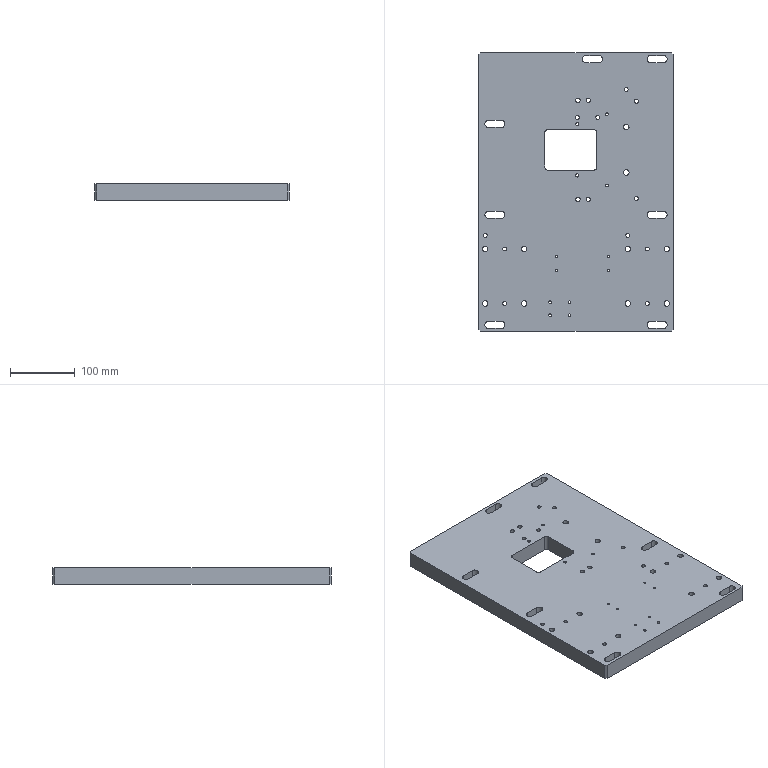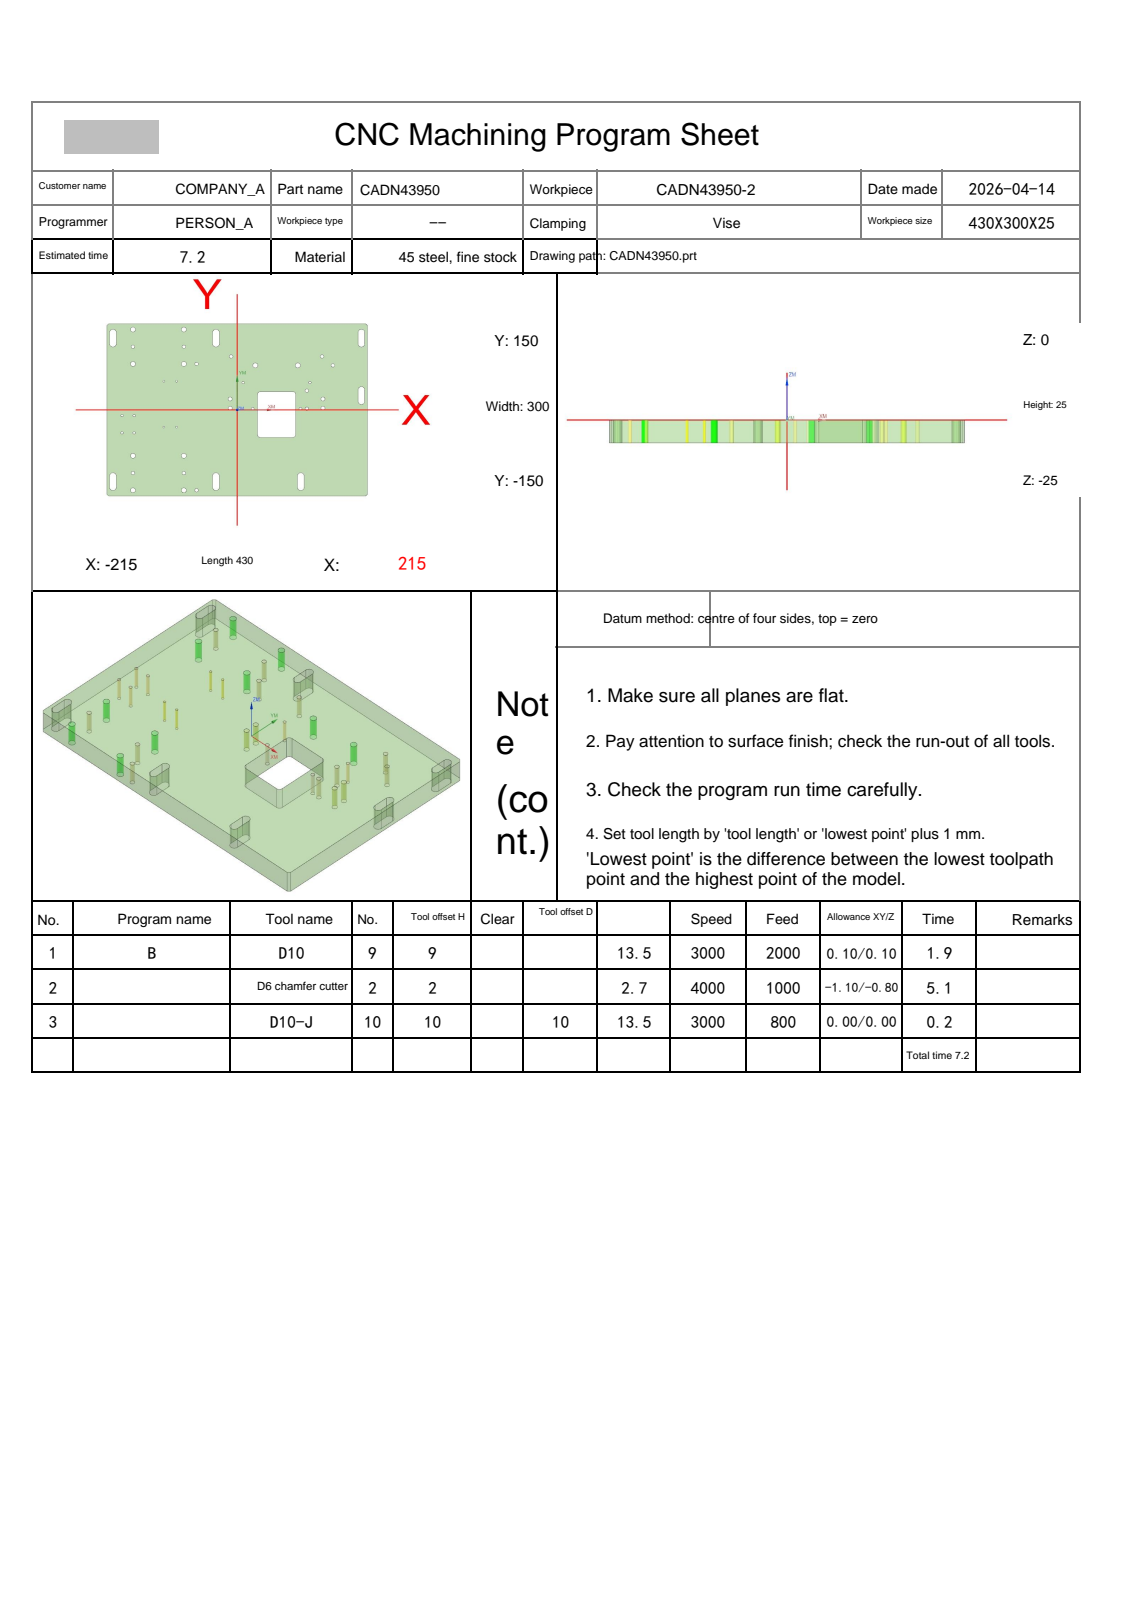NC program | NX | posted by the shop | part box 300 x 430 x 25 mm
Whole program:
%
O0001
(Machine time: 7.60 MIN)
(===Total Tool:3===)
(T9=D10     D=10.  R=0.   D-  H09 Z=-13.5 )
(T2=D6 chamfer cutter D=6. R=0. D- H02 Z=-2.7  )
(T10=D10-J  D=10.  R=0.   D10 H10 Z=-13.5 )
G80 G90 G17 G49 G40
G91 G28 Z0
M01
N1 T09 M06
(D10  D=10. R=0. H=09 ce=0.10 di=0.10)
G00 G90 G54 X-209.112 Y-160.1 M03 S3000
G43 H09 Z20.
M08
Z-.346
G01 X-215.606 Y-153.606 F2000.
X-218.606 Y-150.606
X-225.1 Y-144.112
G00 Z-.692
G01 X-218.606 Y-150.606
X-215.606 Y-153.606
X-209.112 Y-160.1
G00 Z-1.038
G01 X-215.606 Y-153.606
X-218.606 Y-150.606
X-225.1 Y-144.112
G00 Z-1.385
G01 X-218.606 Y-150.606
X-215.606 Y-153.606
X-209.112 Y-160.1
G00 Z-1.731
G01 X-215.606 Y-153.606
X-218.606 Y-150.606
X-225.1 Y-144.112
G00 Z-2.077
G01 X-218.606 Y-150.606
X-215.606 Y-153.606
X-209.112 Y-160.1
G00 Z-2.423
G01 X-215.606 Y-153.606
X-218.606 Y-150.606
X-225.1 Y-144.112
G00 Z-2.769
G01 X-218.606 Y-150.606
X-215.606 Y-153.606
X-209.112 Y-160.1
G00 Z-3.115
G01 X-215.606 Y-153.606
X-218.606 Y-150.606
X-225.1 Y-144.112
G00 Z-3.462
G01 X-218.606 Y-150.606
X-215.606 Y-153.606
X-209.112 Y-160.1
G00 Z-3.808
G01 X-215.606 Y-153.606
X-218.606 Y-150.606
X-225.1 Y-144.112
G00 Z-4.154
G01 X-218.606 Y-150.606
X-215.606 Y-153.606
X-209.112 Y-160.1
G00 Z-4.5
G01 X-215.606 Y-153.606
X-218.606 Y-150.606
X-225.1 Y-144.112
G00 Z-4.846
G01 X-218.606 Y-150.606
X-215.606 Y-153.606
X-209.112 Y-160.1
G00 Z-5.192
G01 X-215.606 Y-153.606
X-218.606 Y-150.606
X-225.1 Y-144.112
G00 Z-5.538
G01 X-218.606 Y-150.606
X-215.606 Y-153.606
X-209.112 Y-160.1
G00 Z-5.885
G01 X-215.606 Y-153.606
X-218.606 Y-150.606
X-225.1 Y-144.112
G00 Z-6.231
G01 X-218.606 Y-150.606
X-215.606 Y-153.606
X-209.112 Y-160.1
G00 Z-6.577
G01 X-215.606 Y-153.606
X-218.606 Y-150.606
X-225.1 Y-144.112
G00 Z-6.923
G01 X-218.606 Y-150.606
X-215.606 Y-153.606
X-209.112 Y-160.1
G00 Z-7.269
G01 X-215.606 Y-153.606
X-218.606 Y-150.606
X-225.1 Y-144.112
G00 Z-7.615
G01 X-218.606 Y-150.606
X-215.606 Y-153.606
X-209.112 Y-160.1
G00 Z-7.962
G01 X-215.606 Y-153.606
X-218.606 Y-150.606
X-225.1 Y-144.112
G00 Z-8.308
G01 X-218.606 Y-150.606
X-215.606 Y-153.606
X-209.112 Y-160.1
G00 Z-8.654
G01 X-215.606 Y-153.606
X-218.606 Y-150.606
X-225.1 Y-144.112
G00 Z-9.
G01 X-218.606 Y-150.606
X-215.606 Y-153.606
X-209.112 Y-160.1
G00 Z-9.346
G01 X-215.606 Y-153.606
X-218.606 Y-150.606
X-225.1 Y-144.112
G00 Z-9.692
G01 X-218.606 Y-150.606
X-215.606 Y-153.606
X-209.112 Y-160.1
G00 Z-10.038
G01 X-215.606 Y-153.606
X-218.606 Y-150.606
X-225.1 Y-144.112
G00 Z-10.385
G01 X-218.606 Y-150.606
X-215.606 Y-153.606
X-209.112 Y-160.1
G00 Z-10.731
G01 X-215.606 Y-153.606
X-218.606 Y-150.606
X-225.1 Y-144.112
G00 Z-11.077
G01 X-218.606 Y-150.606
X-215.606 Y-153.606
X-209.112 Y-160.1
G00 Z-11.423
G01 X-215.606 Y-153.606
X-218.606 Y-150.606
X-225.1 Y-144.112
G00 Z-11.769
G01 X-218.606 Y-150.606
X-215.606 Y-153.606
X-209.112 Y-160.1
G00 Z-12.115
G01 X-215.606 Y-153.606
X-218.606 Y-150.606
X-225.1 Y-144.112
G00 Z-12.462
G01 X-218.606 Y-150.606
X-215.606 Y-153.606
X-209.112 Y-160.1
G00 Z-12.808
G01 X-215.606 Y-153.606
X-218.606 Y-150.606
X-225.1 Y-144.112
G00 Z-13.154
G01 X-218.606 Y-150.606
X-215.606 Y-153.606
X-209.112 Y-160.1
G00 Z-13.5
G01 X-215.606 Y-153.606
X-218.606 Y-150.606
X-225.1 Y-144.112
G00 Z20.
Y144.112
Z-.346
G01 X-218.606 Y150.606
X-215.606 Y153.606
X-209.112 Y160.1
G00 Z-.692
G01 X-215.606 Y153.606
X-218.606 Y150.606
X-225.1 Y144.112
G00 Z-1.038
G01 X-218.606 Y150.606
X-215.606 Y153.606
X-209.112 Y160.1
G00 Z-1.385
G01 X-215.606 Y153.606
X-218.606 Y150.606
X-225.1 Y144.112
G00 Z-1.731
G01 X-218.606 Y150.606
X-215.606 Y153.606
X-209.112 Y160.1
G00 Z-2.077
G01 X-215.606 Y153.606
X-218.606 Y150.606
X-225.1 Y144.112
G00 Z-2.423
G01 X-218.606 Y150.606
X-215.606 Y153.606
X-209.112 Y160.1
G00 Z-2.769
G01 X-215.606 Y153.606
X-218.606 Y150.606
X-225.1 Y144.112
G00 Z-3.115
G01 X-218.606 Y150.606
X-215.606 Y153.606
X-209.112 Y160.1
G00 Z-3.462
G01 X-215.606 Y153.606
X-218.606 Y150.606
X-225.1 Y144.112
G00 Z-3.808
G01 X-218.606 Y150.606
X-215.606 Y153.606
X-209.112 Y160.1
G00 Z-4.154
G01 X-215.606 Y153.606
X-218.606 Y150.606
X-225.1 Y144.112
G00 Z-4.5
G01 X-218.606 Y150.606
X-215.606 Y153.606
X-209.112 Y160.1
G00 Z-4.846
G01 X-215.606 Y153.606
X-218.606 Y150.606
X-225.1 Y144.112
G00 Z-5.192
G01 X-218.606 Y150.606
X-215.606 Y153.606
X-209.112 Y160.1
G00 Z-5.538
G01 X-215.606 Y153.606
X-218.606 Y150.606
X-225.1 Y144.112
G00 Z-5.885
G01 X-218.606 Y150.606
X-215.606 Y153.606
X-209.112 Y160.1
G00 Z-6.231
G01 X-215.606 Y153.606
X-218.606 Y150.606
X-225.1 Y144.112
G00 Z-6.577
G01 X-218.606 Y150.606
X-215.606 Y153.606
X-209.112 Y160.1
G00 Z-6.923
G01 X-215.606 Y153.606
X-218.606 Y150.606
X-225.1 Y144.112
G00 Z-7.269
G01 X-218.606 Y150.606
X-215.606 Y153.606
X-209.112 Y160.1
G00 Z-7.615
G01 X-215.606 Y153.606
X-218.606 Y150.606
X-225.1 Y144.112
G00 Z-7.962
G01 X-218.606 Y150.606
X-215.606 Y153.606
X-209.112 Y160.1
G00 Z-8.308
G01 X-215.606 Y153.606
X-218.606 Y150.606
X-225.1 Y144.112
G00 Z-8.654
G01 X-218.606 Y150.606
X-215.606 Y153.606
X-209.112 Y160.1
G00 Z-9.
G01 X-215.606 Y153.606
X-218.606 Y150.606
X-225.1 Y144.112
G00 Z-9.346
G01 X-218.606 Y150.606
X-215.606 Y153.606
X-209.112 Y160.1
G00 Z-9.692
G01 X-215.606 Y153.606
X-218.606 Y150.606
X-225.1 Y144.112
G00 Z-10.038
G01 X-218.606 Y150.606
X-215.606 Y153.606
X-209.112 Y160.1
G00 Z-10.385
G01 X-215.606 Y153.606
X-218.606 Y150.606
X-225.1 Y144.112
G00 Z-10.731
G01 X-218.606 Y150.606
X-215.606 Y153.606
X-209.112 Y160.1
G00 Z-11.077
G01 X-215.606 Y153.606
X-218.606 Y150.606
X-225.1 Y144.112
G00 Z-11.423
G01 X-218.606 Y150.606
X-215.606 Y153.606
X-209.112 Y160.1
G00 Z-11.769
G01 X-215.606 Y153.606
X-218.606 Y150.606
X-225.1 Y144.112
G00 Z-12.115
G01 X-218.606 Y150.606
X-215.606 Y153.606
X-209.112 Y160.1
G00 Z-12.462
G01 X-215.606 Y153.606
X-218.606 Y150.606
X-225.1 Y144.112
G00 Z-12.808
G01 X-218.606 Y150.606
X-215.606 Y153.606
X-209.112 Y160.1
G00 Z-13.154
G01 X-215.606 Y153.606
X-218.606 Y150.606
X-225.1 Y144.112
G00 Z-13.5
G01 X-218.606 Y150.606
X-215.606 Y153.606
X-209.112 Y160.1
G00 Z20.
X209.112
Z-.346
G01 X215.606 Y153.606
X218.606 Y150.606
X225.1 Y144.112
G00 Z-.692
G01 X218.606 Y150.606
X215.606 Y153.606
X209.112 Y160.1
G00 Z-1.038
G01 X215.606 Y153.606
X218.606 Y150.606
X225.1 Y144.112
G00 Z-1.385
G01 X218.606 Y150.606
X215.606 Y153.606
X209.112 Y160.1
G00 Z-1.731
G01 X215.606 Y153.606
X218.606 Y150.606
X225.1 Y144.112
G00 Z-2.077
G01 X218.606 Y150.606
X215.606 Y153.606
X209.112 Y160.1
G00 Z-2.423
G01 X215.606 Y153.606
X218.606 Y150.606
X225.1 Y144.112
G00 Z-2.769
G01 X218.606 Y150.606
X215.606 Y153.606
X209.112 Y160.1
G00 Z-3.115
G01 X215.606 Y153.606
X218.606 Y150.606
X225.1 Y144.112
G00 Z-3.462
G01 X218.606 Y150.606
X215.606 Y153.606
X209.112 Y160.1
G00 Z-3.808
G01 X215.606 Y153.606
X218.606 Y150.606
X225.1 Y144.112
G00 Z-4.154
G01 X218.606 Y150.606
X215.606 Y153.606
X209.112 Y160.1
G00 Z-4.5
G01 X215.606 Y153.606
X218.606 Y150.606
X225.1 Y144.112
G00 Z-4.846
G01 X218.606 Y150.606
X215.606 Y153.606
X209.112 Y160.1
G00 Z-5.192
G01 X215.606 Y153.606
X218.606 Y150.606
X225.1 Y144.112
G00 Z-5.538
G01 X218.606 Y150.606
X215.606 Y153.606
X209.112 Y160.1
G00 Z-5.885
G01 X215.606 Y153.606
X218.606 Y150.606
X225.1 Y144.112
G00 Z-6.231
G01 X218.606 Y150.606
X215.606 Y153.606
X209.112 Y160.1
G00 Z-6.577
G01 X215.606 Y153.606
X218.606 Y150.606
X225.1 Y144.112
G00 Z-6.923
G01 X218.606 Y150.606
X215.606 Y153.606
X209.112 Y160.1
G00 Z-7.269
G01 X215.606 Y153.606
X218.606 Y150.606
X225.1 Y144.112
G00 Z-7.615
G01 X218.606 Y150.606
X215.606 Y153.606
X209.112 Y160.1
G00 Z-7.962
G01 X215.606 Y153.606
X218.606 Y150.606
X225.1 Y144.112
G00 Z-8.308
G01 X218.606 Y150.606
X215.606 Y153.606
X209.112 Y160.1
G00 Z-8.654
G01 X215.606 Y153.606
X218.606 Y150.606
X225.1 Y144.112
G00 Z-9.
G01 X218.606 Y150.606
X215.606 Y153.606
X209.112 Y160.1
G00 Z-9.346
G01 X215.606 Y153.606
X218.606 Y150.606
X225.1 Y144.112
G00 Z-9.692
G01 X218.606 Y150.606
X215.606 Y153.606
X209.112 Y160.1
G00 Z-10.038
G01 X215.606 Y153.606
X218.606 Y150.606
X225.1 Y144.112
G00 Z-10.385
G01 X218.606 Y150.606
X215.606 Y153.606
X209.112 Y160.1
G00 Z-10.731
G01 X215.606 Y153.606
X218.606 Y150.606
X225.1 Y144.112
G00 Z-11.077
G01 X218.606 Y150.606
X215.606 Y153.606
X209.112 Y160.1
G00 Z-11.423
G01 X215.606 Y153.606
X218.606 Y150.606
X225.1 Y144.112
G00 Z-11.769
G01 X218.606 Y150.606
X215.606 Y153.606
X209.112 Y160.1
G00 Z-12.115
G01 X215.606 Y153.606
X218.606 Y150.606
X225.1 Y144.112
G00 Z-12.462
G01 X218.606 Y150.606
X215.606 Y153.606
X209.112 Y160.1
G00 Z-12.808
G01 X215.606 Y153.606
X218.606 Y150.606
X225.1 Y144.112
G00 Z-13.154
G01 X218.606 Y150.606
X215.606 Y153.606
X209.112 Y160.1
G00 Z-13.5
G01 X215.606 Y153.606
X218.606 Y150.606
X225.1 Y144.112
G00 Z20.
Y-144.112
Z-.346
G01 X218.606 Y-150.606
X215.606 Y-153.606
X209.112 Y-160.1
G00 Z-.692
G01 X215.606 Y-153.606
X218.606 Y-150.606
X225.1 Y-144.112
G00 Z-1.038
G01 X218.606 Y-150.606
X215.606 Y-153.606
X209.112 Y-160.1
G00 Z-1.385
G01 X215.606 Y-153.606
X218.606 Y-150.606
X225.1 Y-144.112
G00 Z-1.731
G01 X218.606 Y-150.606
X215.606 Y-153.606
X209.112 Y-160.1
G00 Z-2.077
G01 X215.606 Y-153.606
X218.606 Y-150.606
X225.1 Y-144.112
G00 Z-2.423
G01 X218.606 Y-150.606
X215.606 Y-153.606
X209.112 Y-160.1
G00 Z-2.769
G01 X215.606 Y-153.606
X218.606 Y-150.606
X225.1 Y-144.112
G00 Z-3.115
G01 X218.606 Y-150.606
X215.606 Y-153.606
X209.112 Y-160.1
G00 Z-3.462
G01 X215.606 Y-153.606
X218.606 Y-150.606
X225.1 Y-144.112
G00 Z-3.808
G01 X218.606 Y-150.606
X215.606 Y-153.606
X209.112 Y-160.1
G00 Z-4.154
G01 X215.606 Y-153.606
X218.606 Y-150.606
X225.1 Y-144.112
G00 Z-4.5
G01 X218.606 Y-150.606
X215.606 Y-153.606
X209.112 Y-160.1
G00 Z-4.846
G01 X215.606 Y-153.606
X218.606 Y-150.606
X225.1 Y-144.112
G00 Z-5.192
G01 X218.606 Y-150.606
X215.606 Y-153.606
X209.112 Y-160.1
G00 Z-5.538
G01 X215.606 Y-153.606
X218.606 Y-150.606
X225.1 Y-144.112
G00 Z-5.885
G01 X218.606 Y-150.606
X215.606 Y-153.606
X209.112 Y-160.1
G00 Z-6.231
G01 X215.606 Y-153.606
X218.606 Y-150.606
X225.1 Y-144.112
G00 Z-6.577
G01 X218.606 Y-150.606
X215.606 Y-153.606
X209.112 Y-160.1
G00 Z-6.923
G01 X215.606 Y-153.606
X218.606 Y-150.606
X225.1 Y-144.112
G00 Z-7.269
G01 X218.606 Y-150.606
X215.606 Y-153.606
X209.112 Y-160.1
G00 Z-7.615
G01 X215.606 Y-153.606
X218.606 Y-150.606
X225.1 Y-144.112
G00 Z-7.962
G01 X218.606 Y-150.606
X215.606 Y-153.606
X209.112 Y-160.1
G00 Z-8.308
G01 X215.606 Y-153.606
X218.606 Y-150.606
X225.1 Y-144.112
G00 Z-8.654
G01 X218.606 Y-150.606
X215.606 Y-153.606
X209.112 Y-160.1
G00 Z-9.
G01 X215.606 Y-153.606
X218.606 Y-150.606
X225.1 Y-144.112
G00 Z-9.346
G01 X218.606 Y-150.606
X215.606 Y-153.606
X209.112 Y-160.1
G00 Z-9.692
G01 X215.606 Y-153.606
X218.606 Y-150.606
X225.1 Y-144.112
G00 Z-10.038
G01 X218.606 Y-150.606
X215.606 Y-153.606
X209.112 Y-160.1
G00 Z-10.385
G01 X215.606 Y-153.606
X218.606 Y-150.606
X225.1 Y-144.112
G00 Z-10.731
G01 X218.606 Y-150.606
X215.606 Y-153.606
X209.112 Y-160.1
G00 Z-11.077
G01 X215.606 Y-153.606
X218.606 Y-150.606
X225.1 Y-144.112
G00 Z-11.423
G01 X218.606 Y-150.606
X215.606 Y-153.606
X209.112 Y-160.1
G00 Z-11.769
G01 X215.606 Y-153.606
X218.606 Y-150.606
X225.1 Y-144.112
G00 Z-12.115
G01 X218.606 Y-150.606
X215.606 Y-153.606
X209.112 Y-160.1
G00 Z-12.462
G01 X215.606 Y-153.606
X218.606 Y-150.606
X225.1 Y-144.112
G00 Z-12.808
G01 X218.606 Y-150.606
X215.606 Y-153.606
X209.112 Y-160.1
G00 Z-13.154
G01 X215.606 Y-153.606
X218.606 Y-150.606
X225.1 Y-144.112
G00 Z-13.5
G01 X218.606 Y-150.606
X215.606 Y-153.606
X209.112 Y-160.1
G00 Z20.
G91 G28 Z0.0
M05
M09
G91 G28 Z0.0
M01
N2 T02 M06
(D6 chamfer cutter D=6. R=0. H=02 ce=0.00 di=0.10)
G00 G90 G54 X-100. Y50. M03 S2000
G43 H02 Z20.
M08
G98 G81 X-100. Y50. Z-2.2 R3. F100.
X-121.
Y-30.
X-100.
G80
G00 Z20.
G00 G90 X-170. Y-40. M03 S2000
Z20.
G98 G81 X-170. Y-40. Z-2.7 R3. F100.
X-190.
Y-10.
X-170.
X10. Y47.5
X120.
G80
G00 Z20.
G00 G90 X105.194 Y2.093 M03 S4000
Z20.
Z-1.1
G01 Z-1.6 F300.
X106. Y2.2
G03 X104.5 Y3.7 I-1.5 J0.0
X102.8 Y2. I0.0 J-1.7
X104.5 Y.3 I1.7 J0.0
X106.2 Y2. I0.0 J1.7
X104.5 Y3.7 I-1.7 J0.0
X103. Y2.2 I0.0 J-1.5
G01 X103.806 Y2.093
Z-1.1
G00 Z20.
X26.194
Z-1.1
G01 Z-1.6
X27. Y2.2
G03 X25.5 Y3.7 I-1.5 J0.0
X23.8 Y2. I0.0 J-1.7
X25.5 Y.3 I1.7 J0.0
X27.2 Y2. I0.0 J1.7
X25.5 Y3.7 I-1.7 J0.0
X24. Y2.2 I0.0 J-1.5
G01 X24.806 Y2.093
Z-1.1
G00 Z20.
G00 G90 X-66.306 Y-139.907 M03 S4000
Z20.
Z-1.1
G01 Z-1.6 F600.
X-65.5 Y-139.8
G03 X-67. Y-138.3 I-1.5 J0.0
X-68.7 Y-140. I0.0 J-1.7
X-67. Y-141.7 I1.7 J0.0
X-65.3 Y-140. I0.0 J1.7
X-67. Y-138.3 I-1.7 J0.0
X-68.5 Y-139.8 I0.0 J-1.5
G01 X-67.694 Y-139.907
Z-1.1
G00 Z20.
X-87.306 Y-109.907
Z-1.1
G01 Z-1.6
X-86.5 Y-109.8
G03 X-88. Y-108.3 I-1.5 J0.0
X-89.7 Y-110. I0.0 J-1.7
X-88. Y-111.7 I1.7 J0.0
X-86.3 Y-110. I0.0 J1.7
X-88. Y-108.3 I-1.7 J0.0
X-89.5 Y-109.8 I0.0 J-1.5
G01 X-88.694 Y-109.907
Z-1.1
G00 Z20.
X-171.306
Z-1.1
G01 Z-1.6
X-170.5 Y-109.8
G03 X-172. Y-108.3 I-1.5 J0.0
X-173.7 Y-110. I0.0 J-1.7
X-172. Y-111.7 I1.7 J0.0
X-170.3 Y-110. I0.0 J1.7
X-172. Y-108.3 I-1.7 J0.0
X-173.5 Y-109.8 I0.0 J-1.5
G01 X-172.694 Y-109.907
Z-1.1
G00 Z20.
X-171.306 Y110.093
Z-1.1
G01 Z-1.6
X-170.5 Y110.2
G03 X-172. Y111.7 I-1.5 J0.0
X-173.7 Y110. I0.0 J-1.7
X-172. Y108.3 I1.7 J0.0
X-170.3 Y110. I0.0 J1.7
X-172. Y111.7 I-1.7 J0.0
X-173.5 Y110.2 I0.0 J-1.5
G01 X-172.694 Y110.093
Z-1.1
G00 Z20.
X-87.306
Z-1.1
G01 Z-1.6
X-86.5 Y110.2
G03 X-88. Y111.7 I-1.5 J0.0
X-89.7 Y110. I0.0 J-1.7
X-88. Y108.3 I1.7 J0.0
X-86.3 Y110. I0.0 J1.7
X-88. Y111.7 I-1.7 J0.0
X-89.5 Y110.2 I0.0 J-1.5
G01 X-88.694 Y110.093
Z-1.1
G00 Z20.
X-66.306 Y80.093
Z-1.1
G01 Z-1.6
X-65.5 Y80.2
G03 X-67. Y81.7 I-1.5 J0.0
X-68.7 Y80. I0.0 J-1.7
X-67. Y78.3 I1.7 J0.0
X-65.3 Y80. I0.0 J1.7
X-67. Y81.7 I-1.7 J0.0
X-68.5 Y80.2 I0.0 J-1.5
G01 X-67.694 Y80.093
Z-1.1
G00 Z20.
X-9.306 Y93.093
Z-1.1
G01 Z-1.6
X-8.5 Y93.2
G03 X-10. Y94.7 I-1.5 J0.0
X-11.7 Y93. I0.0 J-1.7
X-10. Y91.3 I1.7 J0.0
X-8.3 Y93. I0.0 J1.7
X-10. Y94.7 I-1.7 J0.0
X-11.5 Y93.2 I0.0 J-1.5
G01 X-10.694 Y93.093
Z-1.1
G00 Z20.
X140.694
Z-1.1
G01 Z-1.6
X141.5 Y93.2
G03 X140. Y94.7 I-1.5 J0.0
X138.3 Y93. I0.0 J-1.7
X140. Y91.3 I1.7 J0.0
X141.7 Y93. I0.0 J1.7
X140. Y94.7 I-1.7 J0.0
X138.5 Y93.2 I0.0 J-1.5
G01 X139.306 Y93.093
Z-1.1
G00 Z20.
X158.694 Y77.593
Z-1.1
G01 Z-1.6
X159.5 Y77.7
G03 X158. Y79.2 I-1.5 J0.0
X156.3 Y77.5 I0.0 J-1.7
X158. Y75.8 I1.7 J0.0
X159.7 Y77.5 I0.0 J1.7
X158. Y79.2 I-1.7 J0.0
X156.5 Y77.7 I0.0 J-1.5
G01 X157.306 Y77.593
Z-1.1
G00 Z20.
X115.694 Y33.593
Z-1.1
G01 Z-1.6
X116.5 Y33.7
G03 X115. Y35.2 I-1.5 J0.0
X113.3 Y33.5 I0.0 J-1.7
X115. Y31.8 I1.7 J0.0
X116.7 Y33.5 I0.0 J1.7
X115. Y35.2 I-1.7 J0.0
X113.5 Y33.7 I0.0 J-1.5
G01 X114.306 Y33.593
Z-1.1
G00 Z20.
X115.694 Y2.093
Z-1.1
G01 Z-1.6
X116.5 Y2.2
G03 X115. Y3.7 I-1.5 J0.0
X113.3 Y2. I0.0 J-1.7
X115. Y.3 I1.7 J0.0
X116.7 Y2. I0.0 J1.7
X115. Y3.7 I-1.7 J0.0
X113.5 Y2.2 I0.0 J-1.5
G01 X114.306 Y2.093
Z-1.1
G00 Z20.
G00 G90 X-10. Y19.995 M03 S4000
Z20.
Z-1.1
G01 Z-1.6 F300.
Y20.3
G03 X-11.5 Y21.8 I-1.5 J0.0
X-14.3 Y19. I0.0 J-2.8
X-11.5 Y16.2 I2.8 J0.0
X-8.7 Y19. I0.0 J2.8
X-11.5 Y21.8 I-2.8 J0.0
X-13. Y20.3 I0.0 J-1.5
G01 Y19.995
Z-1.1
G00 Z20.
X-10. Y3.995
Z-1.1
G01 Z-1.6
Y4.3
G03 X-11.5 Y5.8 I-1.5 J0.0
X-14.3 Y3. I0.0 J-2.8
X-11.5 Y.2 I2.8 J0.0
X-8.7 Y3. I0.0 J2.8
X-11.5 Y5.8 I-2.8 J0.0
X-13. Y4.3 I0.0 J-1.5
G01 Y3.995
Z-1.1
G00 Z20.
X143.
Z-1.1
G01 Z-1.6
Y4.3
G03 X141.5 Y5.8 I-1.5 J0.0
X138.7 Y3. I0.0 J-2.8
X141.5 Y.2 I2.8 J0.0
X144.3 Y3. I0.0 J2.8
X141.5 Y5.8 I-2.8 J0.0
X140. Y4.3 I0.0 J-1.5
G01 Y3.995
Z-1.1
G00 Z20.
X143. Y19.995
Z-1.1
G01 Z-1.6
Y20.3
G03 X141.5 Y21.8 I-1.5 J0.0
X138.7 Y19. I0.0 J-2.8
X141.5 Y16.2 I2.8 J0.0
X144.3 Y19. I0.0 J2.8
X141.5 Y21.8 I-2.8 J0.0
X140. Y20.3 I0.0 J-1.5
G01 Y19.995
Z-1.1
G00 Z20.
G00 G90 X102.742 Y78.277 M03 S3000
Z20.
Z-1.
G01 Z-1.5 F400.
X103. Y78.35
G03 X100. Y81.35 I-3. J0.0
X96.15 Y77.5 I0.0 J-3.85
X100. Y73.65 I3.85 J0.0
X103.85 Y77.5 I0.0 J3.85
X100. Y81.35 I-3.85 J0.0
X97. Y78.35 I0.0 J-3.
G01 X97.258 Y78.277
Z-1.
G00 Z20.
X32.742
Z-1.
G01 Z-1.5
X33. Y78.35
G03 X30. Y81.35 I-3. J0.0
X26.15 Y77.5 I0.0 J-3.85
X30. Y73.65 I3.85 J0.0
X33.85 Y77.5 I0.0 J3.85
X30. Y81.35 I-3.85 J0.0
X27. Y78.35 I0.0 J-3.
G01 X27.258 Y78.277
Z-1.
G00 Z20.
X-85.258 Y80.777
Z-1.
G01 Z-1.5
X-85. Y80.85
G03 X-88. Y83.85 I-3. J0.0
X-91.85 Y80. I0.0 J-3.85
X-88. Y76.15 I3.85 J0.0
X-84.15 Y80. I0.0 J3.85
X-88. Y83.85 I-3.85 J0.0
X-91. Y80.85 I0.0 J-3.
G01 X-90.742 Y80.777
Z-1.
G00 Z20.
X-85.258 Y140.777
Z-1.
G01 Z-1.5
X-85. Y140.85
G03 X-88. Y143.85 I-3. J0.0
X-91.85 Y140. I0.0 J-3.85
X-88. Y136.15 I3.85 J0.0
X-84.15 Y140. I0.0 J3.85
X-88. Y143.85 I-3.85 J0.0
X-91. Y140.85 I0.0 J-3.
G01 X-90.742 Y140.777
Z-1.
G00 Z20.
X-169.258
Z-1.
G01 Z-1.5
X-169. Y140.85
G03 X-172. Y143.85 I-3. J0.0
X-175.85 Y140. I0.0 J-3.85
X-172. Y136.15 I3.85 J0.0
X-168.15 Y140. I0.0 J3.85
X-172. Y143.85 I-3.85 J0.0
X-175. Y140.85 I0.0 J-3.
G01 X-174.742 Y140.777
Z-1.
G00 Z20.
X-169.258 Y80.777
Z-1.
G01 Z-1.5
X-169. Y80.85
G03 X-172. Y83.85 I-3. J0.0
X-175.85 Y80. I0.0 J-3.85
X-172. Y76.15 I3.85 J0.0
X-168.15 Y80. I0.0 J3.85
X-172. Y83.85 I-3.85 J0.0
X-175. Y80.85 I0.0 J-3.
G01 X-174.742 Y80.777
Z-1.
G00 Z20.
X-169.258 Y-79.223
Z-1.
G01 Z-1.5
X-169. Y-79.15
G03 X-172. Y-76.15 I-3. J0.0
X-175.85 Y-80. I0.0 J-3.85
X-172. Y-83.85 I3.85 J0.0
X-168.15 Y-80. I0.0 J3.85
X-172. Y-76.15 I-3.85 J0.0
X-175. Y-79.15 I0.0 J-3.
G01 X-174.742 Y-79.223
Z-1.
G00 Z20.
X-169.258 Y-139.223
Z-1.
G01 Z-1.5
X-169. Y-139.15
G03 X-172. Y-136.15 I-3. J0.0
X-175.85 Y-140. I0.0 J-3.85
X-172. Y-143.85 I3.85 J0.0
X-168.15 Y-140. I0.0 J3.85
X-172. Y-136.15 I-3.85 J0.0
X-175. Y-139.15 I0.0 J-3.
G01 X-174.742 Y-139.223
Z-1.
G00 Z20.
X-85.258
Z-1.
G01 Z-1.5
X-85. Y-139.15
G03 X-88. Y-136.15 I-3. J0.0
X-91.85 Y-140. I0.0 J-3.85
X-88. Y-143.85 I3.85 J0.0
X-84.15 Y-140. I0.0 J3.85
X-88. Y-136.15 I-3.85 J0.0
X-91. Y-139.15 I0.0 J-3.
G01 X-90.742 Y-139.223
Z-1.
G00 Z20.
X-85.258 Y-79.223
Z-1.
G01 Z-1.5
X-85. Y-79.15
G03 X-88. Y-76.15 I-3. J0.0
X-91.85 Y-80. I0.0 J-3.85
X-88. Y-83.85 I3.85 J0.0
X-84.15 Y-80. I0.0 J3.85
X-88. Y-76.15 I-3.85 J0.0
X-91. Y-79.15 I0.0 J-3.
G01 X-90.742 Y-79.223
Z-1.
G00 Z20.
G00 G90 X-207.743 Y-138.695 M03 S4000
Z20.
Z2.5
G01 X-207.732 Y-138.704 Z2.495 F1000.
X-207.349 Y-138.958 Z2.328
X-206.943 Y-139.173 Z2.16
X-206.517 Y-139.346 Z1.993
X-206.076 Y-139.475 Z1.826
X-205.624 Y-139.56 Z1.658
X-205.166 Y-139.6 Z1.491
X-204.834 Z1.37
X-204.376 Y-139.56 Z1.203
X-203.924 Y-139.475 Z1.035
X-203.483 Y-139.346 Z.868
X-203.057 Y-139.173 Z.701
X-202.651 Y-138.958 Z.534
X-202.268 Y-138.704 Z.366
X-201.912 Y-138.413 Z.199
X-201.587 Y-138.088 Z.032
X-201.296 Y-137.732 Z-.136
X-201.042 Y-137.349 Z-.303
X-200.827 Y-136.943 Z-.47
X-200.654 Y-136.517 Z-.638
X-200.525 Y-136.076 Z-.805
X-200.44 Y-135.624 Z-.972
X-200.4 Y-135.166 Z-1.14
Y-135. Z-1.2
Y-115.
G03 X-205. Y-110.4 I-4.6 J0.0
X-209.6 Y-115. I0.0 J-4.6
G01 Y-135.
G03 X-205. Y-139.6 I4.6 J0.0
X-200.4 Y-135. I0.0 J4.6
G01 Y-134.5
Z1.3
G00 Z20.
X-37.743 Y-138.695
Z2.5
G01 X-37.732 Y-138.704 Z2.495
X-37.349 Y-138.958 Z2.328
X-36.943 Y-139.173 Z2.16
X-36.517 Y-139.346 Z1.993
X-36.076 Y-139.475 Z1.826
X-35.624 Y-139.56 Z1.658
X-35.166 Y-139.6 Z1.491
X-34.834 Z1.37
X-34.376 Y-139.56 Z1.203
X-33.924 Y-139.475 Z1.035
X-33.483 Y-139.346 Z.868
X-33.057 Y-139.173 Z.701
X-32.651 Y-138.958 Z.534
X-32.268 Y-138.704 Z.366
X-31.912 Y-138.413 Z.199
X-31.587 Y-138.088 Z.032
X-31.296 Y-137.732 Z-.136
X-31.042 Y-137.349 Z-.303
X-30.827 Y-136.943 Z-.47
X-30.654 Y-136.517 Z-.638
X-30.525 Y-136.076 Z-.805
X-30.44 Y-135.624 Z-.972
X-30.4 Y-135.166 Z-1.14
Y-135. Z-1.2
Y-115.
G03 X-35. Y-110.4 I-4.6 J0.0
X-39.6 Y-115. I0.0 J-4.6
G01 Y-135.
G03 X-35. Y-139.6 I4.6 J0.0
X-30.4 Y-135. I0.0 J4.6
G01 Y-134.5
Z1.3
G00 Z20.
X102.257 Y-138.695
Z2.5
G01 X102.268 Y-138.704 Z2.495
X102.651 Y-138.958 Z2.328
X103.057 Y-139.173 Z2.16
X103.483 Y-139.346 Z1.993
X103.924 Y-139.475 Z1.826
X104.376 Y-139.56 Z1.658
X104.834 Y-139.6 Z1.491
X105.166 Z1.37
X105.624 Y-139.56 Z1.203
X106.076 Y-139.475 Z1.035
X106.517 Y-139.346 Z.868
X106.943 Y-139.173 Z.701
X107.349 Y-138.958 Z.534
X107.732 Y-138.704 Z.366
X108.088 Y-138.413 Z.199
X108.413 Y-138.088 Z.032
X108.704 Y-137.732 Z-.136
X108.958 Y-137.349 Z-.303
X109.173 Y-136.943 Z-.47
X109.346 Y-136.517 Z-.638
X109.475 Y-136.076 Z-.805
X109.56 Y-135.624 Z-.972
X109.6 Y-135.166 Z-1.14
Y-135. Z-1.2
Y-115.
G03 X105. Y-110.4 I-4.6 J0.0
X100.4 Y-115. I0.0 J-4.6
G01 Y-135.
G03 X105. Y-139.6 I4.6 J0.0
X109.6 Y-135. I0.0 J4.6
G01 Y-134.5
Z1.3
G00 Z20.
X202.257 Y11.305
Z2.5
G01 X202.268 Y11.296 Z2.495
X202.651 Y11.042 Z2.328
X203.057 Y10.827 Z2.16
X203.483 Y10.654 Z1.993
X203.924 Y10.525 Z1.826
X204.376 Y10.44 Z1.658
X204.834 Y10.4 Z1.491
X205.166 Z1.37
X205.624 Y10.44 Z1.203
X206.076 Y10.525 Z1.035
X206.517 Y10.654 Z.868
X206.943 Y10.827 Z.701
X207.349 Y11.042 Z.534
X207.732 Y11.296 Z.366
X208.088 Y11.587 Z.199
X208.413 Y11.912 Z.032
X208.704 Y12.268 Z-.136
X208.958 Y12.651 Z-.303
X209.173 Y13.057 Z-.47
X209.346 Y13.483 Z-.638
X209.475 Y13.924 Z-.805
X209.56 Y14.376 Z-.972
X209.6 Y14.834 Z-1.14
Y15. Z-1.2
Y35.
G03 X205. Y39.6 I-4.6 J0.0
X200.4 Y35. I0.0 J-4.6
G01 Y15.
G03 X205. Y10.4 I4.6 J0.0
X209.6 Y15. I0.0 J4.6
G01 Y15.5
Z1.3
G00 Z20.
X202.257 Y111.305
Z2.5
G01 X202.268 Y111.296 Z2.495
X202.651 Y111.042 Z2.328
X203.057 Y110.827 Z2.16
X203.483 Y110.654 Z1.993
X203.924 Y110.525 Z1.826
X204.376 Y110.44 Z1.658
X204.834 Y110.4 Z1.491
X205.166 Z1.37
X205.624 Y110.44 Z1.203
X206.076 Y110.525 Z1.035
X206.517 Y110.654 Z.868
X206.943 Y110.827 Z.701
X207.349 Y111.042 Z.534
X207.732 Y111.296 Z.366
X208.088 Y111.587 Z.199
X208.413 Y111.912 Z.032
X208.704 Y112.268 Z-.136
X208.958 Y112.651 Z-.303
X209.173 Y113.057 Z-.47
X209.346 Y113.483 Z-.638
X209.475 Y113.924 Z-.805
X209.56 Y114.376 Z-.972
X209.6 Y114.834 Z-1.14
Y115. Z-1.2
Y135.
G03 X205. Y139.6 I-4.6 J0.0
X200.4 Y135. I0.0 J-4.6
G01 Y115.
G03 X205. Y110.4 I4.6 J0.0
X209.6 Y115. I0.0 J4.6
G01 Y115.5
Z1.3
G00 Z20.
X81.334 Y-47.1
Z2.5
G01 X91.5 Z-1.2
G03 X95.6 Y-43. I0.0 J4.1
G01 Y27.
G03 X91.5 Y31.1 I-4.1 J0.0
G01 X38.5
G03 X34.4 Y27. I0.0 J-4.1
G01 Y-43.
G03 X38.5 Y-47.1 I4.1 J0.0
G01 X91.5
G03 X91.999 Y-47.07 I0.0 J4.1
G01 Z1.3
G00 Z20.
X-202.654 Y-150.9
Z2.5
G01 X-211.876 Z-.856
X-211.961 Z-.887
X-212.152 Y-150.871 Z-.958
X-212.336 Y-150.811 Z-1.028
X-212.508 Y-150.723 Z-1.099
X-212.664 Y-150.609 Z-1.169
X-212.724 Y-150.549 Z-1.2
X-215.549 Y-147.724
G02 X-215.9 Y-146.876 I.849 J.849
G01 Y146.876
G02 X-215.549 Y147.724 I1.2 J0.0
G01 X-212.724 Y150.549
G02 X-211.876 Y150.9 I.849 J-.849
G01 X211.876
G02 X212.724 Y150.549 I0.0 J-1.2
G01 X215.549 Y147.724
G02 X215.9 Y146.876 I-.849 J-.849
G01 Y-146.876
G02 X215.549 Y-147.724 I-1.2 J0.0
G01 X212.724 Y-150.549
G02 X211.876 Y-150.9 I-.849 J.849
G01 X-211.876
G02 X-212.724 Y-150.549 I0.0 J1.2
G01 X-213.078 Y-150.195
Z1.3
G00 Z20.
X-37.743 Y111.305
Z2.5
G01 X-37.732 Y111.296 Z2.495
X-37.349 Y111.042 Z2.328
X-36.943 Y110.827 Z2.16
X-36.517 Y110.654 Z1.993
X-36.076 Y110.525 Z1.826
X-35.624 Y110.44 Z1.658
X-35.166 Y110.4 Z1.491
X-34.834 Z1.37
X-34.376 Y110.44 Z1.203
X-33.924 Y110.525 Z1.035
X-33.483 Y110.654 Z.868
X-33.057 Y110.827 Z.701
X-32.651 Y111.042 Z.534
X-32.268 Y111.296 Z.366
X-31.912 Y111.587 Z.199
X-31.587 Y111.912 Z.032
X-31.296 Y112.268 Z-.136
X-31.042 Y112.651 Z-.303
X-30.827 Y113.057 Z-.47
X-30.654 Y113.483 Z-.638
X-30.525 Y113.924 Z-.805
X-30.44 Y114.376 Z-.972
X-30.4 Y114.834 Z-1.14
Y115. Z-1.2
Y135.
G03 X-35. Y139.6 I-4.6 J0.0
X-39.6 Y135. I0.0 J-4.6
G01 Y115.
G03 X-35. Y110.4 I4.6 J0.0
X-30.4 Y115. I0.0 J4.6
G01 Y115.5
Z1.3
G00 Z20.
X-207.743 Y111.305
Z2.5
G01 X-207.732 Y111.296 Z2.495
X-207.349 Y111.042 Z2.328
X-206.943 Y110.827 Z2.16
X-206.517 Y110.654 Z1.993
X-206.076 Y110.525 Z1.826
X-205.624 Y110.44 Z1.658
X-205.166 Y110.4 Z1.491
X-204.834 Z1.37
X-204.376 Y110.44 Z1.203
X-203.924 Y110.525 Z1.035
X-203.483 Y110.654 Z.868
X-203.057 Y110.827 Z.701
X-202.651 Y111.042 Z.534
X-202.268 Y111.296 Z.366
X-201.912 Y111.587 Z.199
X-201.587 Y111.912 Z.032
X-201.296 Y112.268 Z-.136
X-201.042 Y112.651 Z-.303
X-200.827 Y113.057 Z-.47
X-200.654 Y113.483 Z-.638
X-200.525 Y113.924 Z-.805
X-200.44 Y114.376 Z-.972
X-200.4 Y114.834 Z-1.14
Y115. Z-1.2
Y135.
G03 X-205. Y139.6 I-4.6 J0.0
X-209.6 Y135. I0.0 J-4.6
G01 Y115.
G03 X-205. Y110.4 I4.6 J0.0
X-200.4 Y115. I0.0 J4.6
G01 Y115.5
Z1.3
G00 Z20.
G91 G28 Z0.0
M05
M09
G91 G28 Z0.0
M01
N3 T10 M06
(D10-J  D=10. R=0. H=10 ce=0.00 di=0.00)
G00 G90 G54 X220.684 Y-150.544 M03 S3000
G43 H10 Z5.
M08
Z-12.5
G01 Z-13.5 F800.
G41 D10
X220.527 Y-150.42
G03 X219.596 Y-150.096 I-.931 J-1.176
X218.536 Y-150.536 I0.0 J-1.5
G01 X215.536 Y-153.536
G03 X215.096 Y-154.596 I1.061 J-1.061
X215.42 Y-155.527 I1.5 J0.0
G01 G40 X215.544 Y-155.684
Z-12.5
G00 Z5.
Y155.684
Z-12.5
G01 Z-13.5
G41 D10
X215.42 Y155.527
G03 X215.096 Y154.596 I1.176 J-.931
X215.536 Y153.536 I1.5 J0.0
G01 X218.536 Y150.536
G03 X219.596 Y150.096 I1.061 J1.061
X220.527 Y150.42 I0.0 J1.5
G01 G40 X220.684 Y150.544
Z-12.5
G00 Z5.
X-220.684
Z-12.5
G01 Z-13.5
G41 D10
X-220.527 Y150.42
G03 X-219.596 Y150.096 I.931 J1.176
X-218.536 Y150.536 I0.0 J1.5
G01 X-215.536 Y153.536
G03 X-215.096 Y154.596 I-1.061 J1.061
X-215.42 Y155.527 I-1.5 J0.0
G01 G40 X-215.544 Y155.684
Z-12.5
G00 Z5.
Y-155.684
Z-12.5
G01 Z-13.5
G41 D10
X-215.42 Y-155.527
G03 X-215.096 Y-154.596 I-1.176 J.931
X-215.536 Y-153.536 I-1.5 J0.0
G01 X-218.536 Y-150.536
G03 X-219.596 Y-150.096 I-1.061 J-1.061
X-220.527 Y-150.42 I0.0 J-1.5
G01 G40 X-220.684 Y-150.544
Z-12.5
G00 Z5.
M05
M09
G91 G28 Z0.0
G91 G28 Y0.0
M30
%